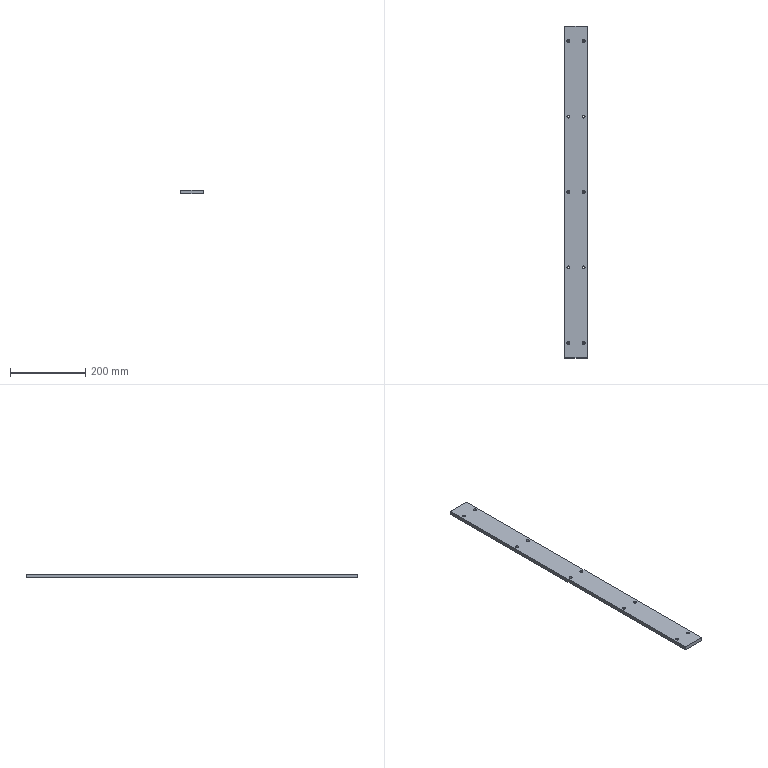Part | STEP file | LIFT.PAD.2.stp | 1 solid | 56 faces | box 60 x 880 x 10 mm | volume 524898 mm3 | spline 25 | cylinder 24 | plane 7 | commonest cylinder face diameters 4.5 x12 8 x12